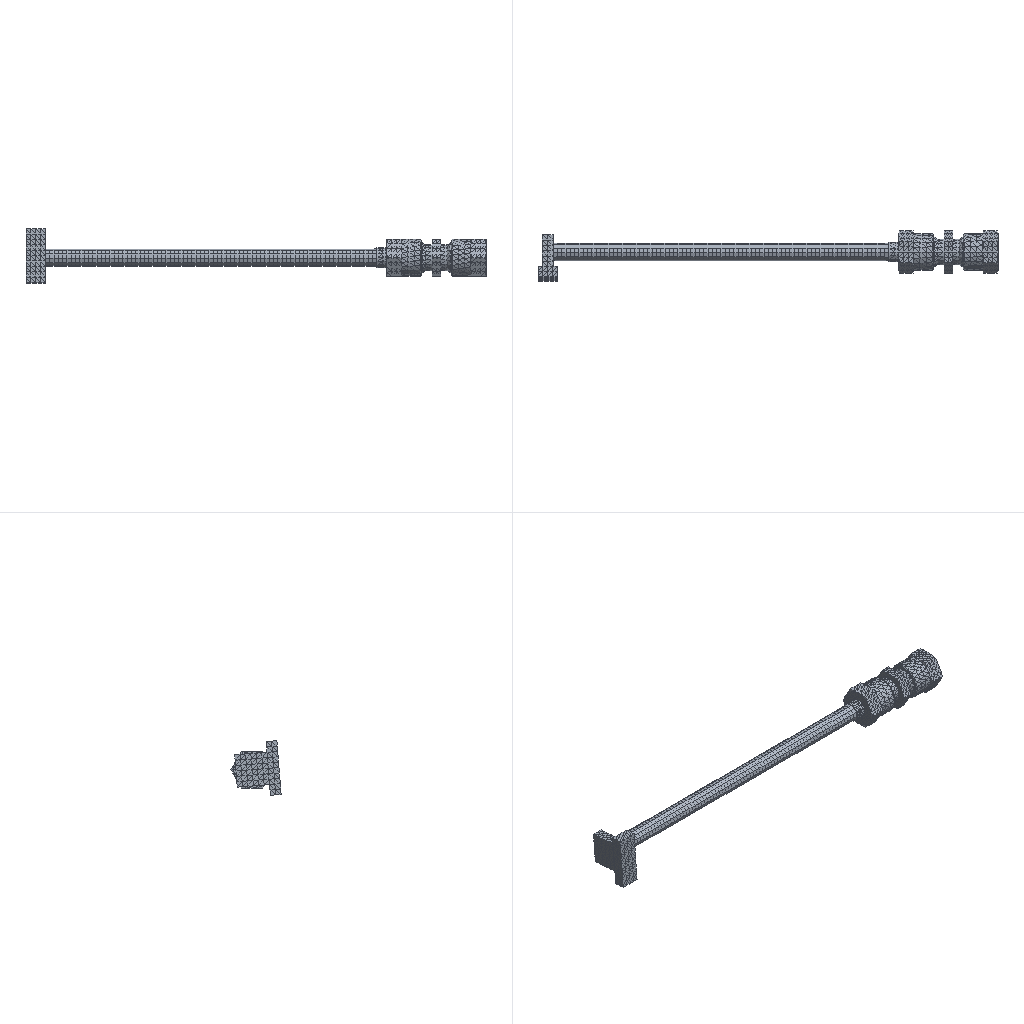Simulation study | abaqus
Set-up summary:
category,name,step,type,value,unit,region
solver,abaqus,,Abaqus/CAE 2024
units,mm-N-s-tonne (MPa),,inferred,E=106000 density=4.48e-09
analysis,Step-1,,static,time_period=1
mesh,nodes,,,14303
mesh,elements,,,7999
element_type,C3D10,,,6919
element_type,S4R,,,1080
material,dg,,E,106000
material,dg,,nu,0.3
material,dg,,density,4.48e-09
material,dg,,cte,8.3e-06
material,dg,,behaviors,expansion
material,jt,,E,119000
material,jt,,nu,0.34
material,jt,,density,4.5e-09
material,jt,,cte,8.2e-06
material,jt,,behaviors,expansion
section,jt,,solid section,,,Set-1
section,jt,,solid section,,,Set-1
section,jt,,solid section,,,Set-1
section,jt,,solid section,,,Set-1
section,jt,,solid section,,,Set-1
section,jt,,solid section,,,Set-1
section,dg,,shell section,0.54,,Set-2
load,Predefined,initial,initial condition temperature
load,Load-1,Step-1,pressure,35,,Surf-13
load,Load-2,Step-1,pressure,35,,Surf-14
load,Predefined,Step-1,temperature,50,,Set-2
bc,BC-1,Step-1,encastre,[dofs=ENCASTRE],,Set-1
contact,Constraint-1,initial,tie,,,s_Surf-1 / m_Surf-1
contact,Constraint-2,initial,tie,,,s_Surf-3 / m_Surf-3
contact,Constraint-3,initial,tie,,,s_Surf-5 / m_Surf-5
contact,Constraint-4,initial,tie,,,s_Surf-7 / m_Surf-7
contact,Constraint-5,initial,tie,,,s_Surf-9 / m_Surf-9
contact,Constraint-6,initial,tie,,,s_Surf-11 / m_Surf-11
Abaqus input file, long lists of numbers shortened:
*Heading
** Job name: deck Model name: Model-1
** Generated by: Abaqus/CAE 2024
*Preprint, echo=NO, model=NO, history=NO, contact=NO
**
** PARTS
**
*Part, name=dg
*End Part
**
*Part, name=gt
*Node
      1,  -21.082, -0.3744,          -6.
      2,  -15.858, -0.3744,          -6.
** (1643 more lines like these left out)
*Element, type=C3D10
  1,  245,   91,  111,   92,  286,  285,  284,  288,  287,  289
  2,  246,  245,  110,  134,  292,  291,  290,  294,  293,  295
** (815 more lines like these left out)
*Nset, nset=Set-1, generate
    1,  1645,     1
*Elset, elset=Set-1, generate
   1,  817,    1
** Section: jt
*Solid Section, elset=Set-1, material=jt
,
*End Part
**
*Part, name=jiaju
*Node
      1,  -190.749,  -13.813,  -11.485
      2,  -181.749,  -13.813,  -11.485
** (2282 more lines like these left out)
*Element, type=C3D10
   1,  119,  262,  263,  252,  368,  367,  366,  370,  369,  371
   2,  181,  262,  219,  264,  374,  373,  372,  376,  375,  377
** (1294 more lines like these left out)
*Nset, nset=Set-1, generate
    1,  2284,     1
*Elset, elset=Set-1, generate
    1,  1296,     1
** Section: jt
*Solid Section, elset=Set-1, material=jt
,
*End Part
**
*Part, name=jietouzuo
*Node
      1,  -5.749, -0.3744,  -5.95
      2,  -5.749, -0.3744,   5.95
** (1310 more lines like these left out)
*Element, type=C3D10
  1,  187,   68,  104,  166,  221,  220,  219,  223,  222,  224
  2,  187,  103,   68,   67,  226,  225,  221,  228,  227,  229
** (688 more lines like these left out)
*Nset, nset=Set-1, generate
    1,  1312,     1
*Elset, elset=Set-1, generate
   1,  690,    1
** Section: jt
*Solid Section, elset=Set-1, material=jt
,
*End Part
**
*Part, name=jtyou
*Node
      1,   10.751, -0.3744,           7.
      2,   5.751, -0.3744,           7.
** (2225 more lines like these left out)
*Element, type=C3D10
   1,  309,  287,  310,  311,  368,  367,  366,  370,  369,  371
   2,  309,  257,   15,  164,  374,  373,  372,  376,  375,  377
** (1187 more lines like these left out)
*Nset, nset=Set-1, generate
    1,  2227,     1
*Elset, elset=Set-1, generate
    1,  1189,     1
** Section: jt
*Solid Section, elset=Set-1, material=jt
,
*End Part
**
*Part, name=lmyou
*Node
      1,   22.11, -0.3744,        4.625
      2,   22.11, -0.3744,       -4.625
** (2978 more lines like these left out)
*Element, type=C3D10
   1,  460,  461,   79,  295,  499,  498,  497,  501,  500,  502
   2,  460,  462,  276,   80,  505,  504,  503,  507,  506,  508
** (1530 more lines like these left out)
*Nset, nset=Set-1, generate
    1,  2980,     1
*Elset, elset=Set-1, generate
    1,  1532,     1
** Section: jt
*Solid Section, elset=Set-1, material=jt
,
*End Part
**
*Part, name=lmzuo
*Node
      1,  -23.607, -0.3744,        4.625
      2,  -23.607, -0.3744,       -4.625
** (2761 more lines like these left out)
*Element, type=C3D10
   1,  435,  436,   94,  279,  470,  469,  468,  472,  471,  473
   2,  162,  308,  200,  437,  476,  475,  474,  478,  477,  479
** (1393 more lines like these left out)
*Nset, nset=Set-1, generate
    1,  2763,     1
*Elset, elset=Set-1, generate
    1,  1395,     1
** Section: jt
*Solid Section, elset=Set-1, material=jt
,
*End Part
**
**
** ASSEMBLY
**
*Assembly, name=Assembly
**
*Instance, name=dg-1, part=dg
*Node
      1,  -12.308, -0.7027,   3.986
      2,  -12.308, -0.046,  -3.986
** (1090 more lines like these left out)
*Element, type=S4R
 1,   1,  11, 233,  22
 2,  11,  12, 234, 233
** (1078 more lines like these left out)
*Nset, nset=Set-2, generate
    1,  1092,     1
*Elset, elset=Set-2, generate
    1,  1080,     1
** Section: dg
*Shell Section, elset=Set-2, material=dg, offset=SPOS
0.54, 5
*End Instance
**
*Instance, name=gt-1, part=gt
*End Instance
**
*Instance, name=jiaju-1, part=jiaju
*End Instance
**
*Instance, name=jietouzuo-1, part=jietouzuo
*End Instance
**
*Instance, name=jtyou-1, part=jtyou
*End Instance
**
*Instance, name=lmyou-1, part=lmyou
*End Instance
**
*Instance, name=lmzuo-1, part=lmzuo
*End Instance
**
*Nset, nset=Set-1, instance=jiaju-1
    1,    2,    3,    4,   21,   22,   23,   24,   25,   26,   27,   28,   29,   30,   31,   32
   33,   34,   35,   36,   37,   38,   39,   40,   41,   42,   43,   44,  135,  136,  137,  138
** (10 more lines like these left out)
*Elset, elset=Set-1, instance=jiaju-1
   29,   42,   79,   80,  112,  129,  168,  207,  242,  266,  271,  274,  284,  297,  300,  331
  341,  356,  399,  416,  446,  448,  464,  493,  531,  592,  631,  640,  691,  693,  697,  712
** (3 more lines like these left out)
*Nset, nset=Set-2, instance=dg-1, generate
    1,  1092,     1
*Nset, nset=Set-2, instance=gt-1, generate
    1,  1645,     1
*Nset, nset=Set-2, instance=jietouzuo-1, generate
    1,  1312,     1
*Nset, nset=Set-2, instance=lmyou-1, generate
    1,  2980,     1
*Nset, nset=Set-2, instance=jiaju-1, generate
    1,  2284,     1
*Nset, nset=Set-2, instance=jtyou-1, generate
    1,  2227,     1
*Elset, elset=Set-2, instance=dg-1, generate
    1,  1080,     1
*Elset, elset=Set-2, instance=gt-1, generate
   1,  817,    1
*Elset, elset=Set-2, instance=jietouzuo-1, generate
   1,  690,    1
*Elset, elset=Set-2, instance=lmyou-1, generate
    1,  1532,     1
*Elset, elset=Set-2, instance=jiaju-1, generate
    1,  1296,     1
*Elset, elset=Set-2, instance=jtyou-1, generate
    1,  1189,     1
*Nset, nset=Set-3, instance=dg-1, generate
    1,  1092,     1
*Nset, nset=Set-3, instance=gt-1, generate
    1,  1645,     1
*Nset, nset=Set-3, instance=jietouzuo-1, generate
    1,  1312,     1
*Nset, nset=Set-3, instance=lmyou-1, generate
    1,  2980,     1
*Nset, nset=Set-3, instance=jiaju-1, generate
    1,  2284,     1
*Nset, nset=Set-3, instance=jtyou-1, generate
    1,  2227,     1
*Elset, elset=Set-3, instance=dg-1, generate
    1,  1080,     1
*Elset, elset=Set-3, instance=gt-1, generate
   1,  817,    1
*Elset, elset=Set-3, instance=jietouzuo-1, generate
   1,  690,    1
*Elset, elset=Set-3, instance=lmyou-1, generate
    1,  1532,     1
*Elset, elset=Set-3, instance=jiaju-1, generate
    1,  1296,     1
*Elset, elset=Set-3, instance=jtyou-1, generate
    1,  1189,     1
*Elset, elset=_Surf-13_SNEG, internal, instance=dg-1, generate
    1,  1080,     1
*Surface, type=ELEMENT, name=Surf-13
_Surf-13_SNEG, SNEG
*Elset, elset=_Surf-14_S3, internal, instance=jietouzuo-1
  26,  52,  83,  91, 127, 192, 202, 304, 406, 438, 542, 565, 566, 574, 581, 585
 586, 589, 591, 592, 598, 620, 666, 668, 689
*Elset, elset=_Surf-14_S3, internal, instance=jtyou-1
   19,   20,  177,  207,  227,  350,  353,  361,  400,  421,  499,  505,  513,  515,  523,  524
  526,  536,  553,  561,  562,  578,  596,  598,  675,  688,  691,  768,  872,  944,  993, 1002
** (1 more lines like these left out)
*Elset, elset=_Surf-14_S2, internal, instance=jietouzuo-1
 432, 434, 482, 634, 637
*Elset, elset=_Surf-14_S2, internal, instance=jtyou-1
  238,  482,  597,  721,  725,  771, 1136, 1181
*Elset, elset=_Surf-14_S4, internal, instance=jietouzuo-1
 535,
*Elset, elset=_Surf-14_S4, internal, instance=jtyou-1
  289,  415,  425,  504,  551,  552,  554,  574,  603,  971,  983, 1095
*Elset, elset=_Surf-14_S1, internal, instance=jietouzuo-1
 416,
*Elset, elset=_Surf-14_S1, internal, instance=jtyou-1
  516,  518,  713,  758,  831, 1093, 1119, 1122
*Surface, type=ELEMENT, name=Surf-14
_Surf-14_S3, S3
_Surf-14_S2, S2
_Surf-14_S4, S4
_Surf-14_S1, S1
*Elset, elset=_m_Surf-1_S3, internal, instance=jiaju-1
  101,  110,  375,  435,  472,  522,  620,  723,  730,  746,  750,  752,  756,  764,  774,  779
  825,  831,  892,  957,  992, 1182
*Elset, elset=_m_Surf-1_S2, internal, instance=jiaju-1
  114,  731,  771,  800,  832, 1128
*Elset, elset=_m_Surf-1_S1, internal, instance=jiaju-1
    5,  188,  776,  777,  787,  812,  933, 1035, 1199
*Elset, elset=_m_Surf-1_S4, internal, instance=jiaju-1
  790,  983, 1065
*Surface, type=ELEMENT, name=m_Surf-1
_m_Surf-1_S3, S3
_m_Surf-1_S2, S2
_m_Surf-1_S4, S4
_m_Surf-1_S1, S1
*Elset, elset=_m_Surf-3_S1, internal, instance=lmzuo-1
   63,  177,  209,  214,  243,  269,  295,  301,  379,  396,  441,  453,  462,  471,  497,  502
  519,  534,  543,  560,  569,  579,  590,  594,  607,  628,  664,  679,  688,  706,  708,  785
** (1 more lines like these left out)
*Elset, elset=_m_Surf-3_S4, internal, instance=lmzuo-1
  213,  265,  267,  279,  300,  312,  361,  430,  447,  459,  460,  492,  512,  516,  518,  523
  531,  538,  539,  549,  552,  558,  559,  565,  566,  567,  606,  641,  657,  701,  714,  743
** (1 more lines like these left out)
*Elset, elset=_m_Surf-3_S2, internal, instance=lmzuo-1
  197,  227,  235,  247,  284,  286,  299,  330,  350,  424,  439,  456,  465,  489,  520,  581
  585,  597,  608,  609,  610,  617,  622,  626,  635,  687,  700,  709,  720,  754,  767,  801
** (1 more lines like these left out)
*Elset, elset=_m_Surf-3_S3, internal, instance=lmzuo-1
  184,  296,  318,  336,  340,  353,  390,  393,  394,  403,  404,  405,  406,  423,  428,  436
  446,  450,  467,  470,  475,  480,  483,  490,  499,  507,  550,  551,  573,  574,  587,  598
** (2 more lines like these left out)
*Surface, type=ELEMENT, name=m_Surf-3
_m_Surf-3_S1, S1
_m_Surf-3_S4, S4
_m_Surf-3_S2, S2
_m_Surf-3_S3, S3
*Elset, elset=_m_Surf-5_S3, internal, instance=lmyou-1
   74,  253,  254,  260,  262,  330,  334,  345,  364,  368,  375,  382,  416,  422,  432,  439
  440,  447,  452,  457,  461,  508,  560,  562,  573,  590,  591,  599,  602,  679,  681,  708
** (1 more lines like these left out)
*Elset, elset=_m_Surf-5_S2, internal, instance=lmyou-1
  247,  276,  279,  307,  309,  366,  373,  398,  413,  417,  418,  453,  466,  472,  474,  480
  485,  498,  506,  523,  540,  545,  567,  570,  575,  576,  611,  631,  639,  664,  754,  765
** (1 more lines like these left out)
*Elset, elset=_m_Surf-5_S4, internal, instance=lmyou-1
  255,  264,  311,  326,  333,  377,  378,  384,  389,  391,  393,  406,  410,  411,  423,  437
  442,  454,  460,  467,  479,  487,  489,  494,  510,  512,  527,  533,  539,  549,  574,  589
** (2 more lines like these left out)
*Elset, elset=_m_Surf-5_S1, internal, instance=lmyou-1
   82,  207,  244,  267,  275,  290,  337,  342,  347,  394,  455,  491,  502,  505,  513,  518
  526,  535,  544,  565,  566,  569,  578,  582,  588,  675,  734,  750,  789,  841,  867,  907
** (1 more lines like these left out)
*Surface, type=ELEMENT, name=m_Surf-5
_m_Surf-5_S3, S3
_m_Surf-5_S2, S2
_m_Surf-5_S4, S4
_m_Surf-5_S1, S1
*Elset, elset=_m_Surf-7_S4, internal, instance=jietouzuo-1
  14,  48, 177, 204, 285, 291, 324
*Elset, elset=_m_Surf-7_S3, internal, instance=jietouzuo-1
  21,  74,  85, 156, 173, 185, 206, 235, 240, 242, 244, 252, 298, 300, 306, 339
 362, 408, 452, 604, 622
*Elset, elset=_m_Surf-7_S1, internal, instance=jietouzuo-1
  30, 258, 316, 331
*Elset, elset=_m_Surf-7_S2, internal, instance=jietouzuo-1
 241, 325, 357, 522
*Surface, type=ELEMENT, name=m_Surf-7
_m_Surf-7_S4, S4
_m_Surf-7_S3, S3
_m_Surf-7_S2, S2
_m_Surf-7_S1, S1
*Elset, elset=_m_Surf-9_S2, internal, instance=gt-1
   3,  46,  60,  65, 109, 113, 123, 135, 157, 172, 176, 199, 203, 208, 231, 240
 244, 259, 315, 321, 348, 367, 380, 383, 398, 573, 592, 644
*Elset, elset=_m_Surf-9_S4, internal, instance=gt-1
   4,  17,  40,  70,  72,  95, 100, 107, 130, 133, 137, 161, 221, 224, 238, 239
 264, 290, 303, 330, 392, 407, 425, 427, 475, 485, 543, 657, 675, 697, 704, 710
** (1 more lines like these left out)
*Elset, elset=_m_Surf-9_S1, internal, instance=gt-1
  27,  47,  48,  53,  61,  71,  87,  92, 110, 163, 167, 194, 204, 212, 226, 229
 233, 242, 243, 253, 267, 308, 399, 402, 441, 445, 591, 667, 684, 688, 726
*Elset, elset=_m_Surf-9_S3, internal, instance=gt-1
  34,  42,  58,  84,  96, 105, 126, 140, 153, 162, 170, 180, 183, 191, 200, 213
 214, 230, 249, 260, 295, 325, 338, 451, 629, 680, 683, 706
*Surface, type=ELEMENT, name=m_Surf-9
_m_Surf-9_S2, S2
_m_Surf-9_S4, S4
_m_Surf-9_S1, S1
_m_Surf-9_S3, S3
*Elset, elset=_m_Surf-11_S3, internal, instance=jtyou-1
   59,   81,  127,  135,  170,  174,  190,  254,  277,  282,  285,  297,  298,  303,  341,  346
  351,  374,  406,  416,  428,  433,  435,  440,  448,  449,  452,  460,  465,  482,  493,  503
** (2 more lines like these left out)
*Elset, elset=_m_Surf-11_S2, internal, instance=jtyou-1
  148,  330,  453,  479,  487,  553,  641,  702,  829,  943,  944, 1064
*Elset, elset=_m_Surf-11_S1, internal, instance=jtyou-1
  195,  414,  476,  576,  608,  627,  652,  692, 1168
*Elset, elset=_m_Surf-11_S4, internal, instance=jtyou-1
  387,  446,  455,  494,  505,  520,  536,  566,  632,  651,  653,  670,  695,  735,  968, 1068
*Surface, type=ELEMENT, name=m_Surf-11
_m_Surf-11_S3, S3
_m_Surf-11_S2, S2
_m_Surf-11_S4, S4
_m_Surf-11_S1, S1
*Elset, elset=_s_Surf-1_SPOS, internal, instance=dg-1
 1009, 1010, 1011, 1012, 1013, 1014, 1015, 1016, 1017, 1018, 1019, 1020, 1069, 1070, 1071, 1072
 1073, 1074, 1075, 1076, 1077, 1078, 1079, 1080
*Surface, type=ELEMENT, name=s_Surf-1
_s_Surf-1_SPOS, SPOS
*Elset, elset=_s_Surf-3_S4, internal, instance=jietouzuo-1
   9, 172, 284, 377, 541
*Elset, elset=_s_Surf-3_S3, internal, instance=jietouzuo-1
  60,  65,  66,  97, 107, 110, 111, 129, 134, 149, 151, 178, 181, 205, 261, 272
 278, 327, 332, 340, 343, 369, 371, 404, 428, 431, 436, 444, 465, 466, 473, 480
** (2 more lines like these left out)
*Elset, elset=_s_Surf-3_S1, internal, instance=jietouzuo-1
 157, 174, 247, 260, 262, 269, 472, 494, 627
*Elset, elset=_s_Surf-3_S2, internal, instance=jietouzuo-1
 280, 330, 451, 471, 484, 503
*Surface, type=ELEMENT, name=s_Surf-3
_s_Surf-3_S4, S4
_s_Surf-3_S3, S3
_s_Surf-3_S2, S2
_s_Surf-3_S1, S1
*Elset, elset=_s_Surf-5_S3, internal, instance=jtyou-1
   66,   70,   71,   75,   80,  116,  122,  143,  167,  185,  215,  311,  386,  443,  450,  462
  466,  484,  490,  529,  543,  546,  560,  589,  591,  611,  615,  630,  646,  722,  727,  744
** (2 more lines like these left out)
*Elset, elset=_s_Surf-5_S1, internal, instance=jtyou-1
 137,
*Elset, elset=_s_Surf-5_S4, internal, instance=jtyou-1
  161,  846,  991, 1189
*Elset, elset=_s_Surf-5_S2, internal, instance=jtyou-1
  837,  866, 1129, 1179
*Surface, type=ELEMENT, name=s_Surf-5
_s_Surf-5_S3, S3
_s_Surf-5_S1, S1
_s_Surf-5_S4, S4
_s_Surf-5_S2, S2
*Elset, elset=_s_Surf-7_S3, internal, instance=gt-1
  33,  39, 247, 316, 369, 377
*Elset, elset=_s_Surf-7_S4, internal, instance=gt-1
   8,  28,  37, 252, 255, 553, 586, 672
*Elset, elset=_s_Surf-7_S2, internal, instance=gt-1
 256, 261, 287, 305, 313, 462, 590
*Elset, elset=_s_Surf-7_S1, internal, instance=gt-1
  29, 699, 715
*Surface, type=ELEMENT, name=s_Surf-7
_s_Surf-7_S3, S3
_s_Surf-7_S4, S4
_s_Surf-7_S2, S2
_s_Surf-7_S1, S1
*Elset, elset=_s_Surf-9_SPOS, internal, instance=dg-1
   13,   14,   15,   16,   17,   18,   19,   20,   21,   22,   23,   24,   25,   26,   27,   28
   29,   30,   31,   32,   33,   34,   35,   36,   37,   38,   39,   40,   41,   42,   43,   44
** (4 more lines like these left out)
*Surface, type=ELEMENT, name=s_Surf-9
_s_Surf-9_SPOS, SPOS
*Elset, elset=_s_Surf-11_S4, internal, instance=jietouzuo-1
  25, 672
*Elset, elset=_s_Surf-11_S3, internal, instance=jietouzuo-1
  27,  33, 131, 164, 478, 551, 552, 553, 557, 558, 559, 599, 600, 615, 650, 654
 656, 660, 662, 663, 664, 670, 681
*Elset, elset=_s_Surf-11_S2, internal, instance=jietouzuo-1
 474,
*Surface, type=ELEMENT, name=s_Surf-11
_s_Surf-11_S4, S4
_s_Surf-11_S3, S3
_s_Surf-11_S2, S2
** Constraint: Constraint-1
*Tie, name=Constraint-1, adjust=yes
s_Surf-1, m_Surf-1
** Constraint: Constraint-2
*Tie, name=Constraint-2, adjust=yes
s_Surf-3, m_Surf-3
** Constraint: Constraint-3
*Tie, name=Constraint-3, adjust=yes
s_Surf-5, m_Surf-5
** Constraint: Constraint-4
*Tie, name=Constraint-4, adjust=yes
s_Surf-7, m_Surf-7
** Constraint: Constraint-5
*Tie, name=Constraint-5, adjust=yes
s_Surf-9, m_Surf-9
** Constraint: Constraint-6
*Tie, name=Constraint-6, adjust=yes
s_Surf-11, m_Surf-11
*End Assembly
**
** MATERIALS
**
*Material, name=dg
*Density
 4.48e-09,
*Elastic
106000., 0.3,-55.
104500., 0.3,-20.
103500., 0.3,  0.
101500., 0.3, 50.
 98000., 0.3,100.
 96000., 0.3,120.
 94500., 0.3,135.
 93500., 0.3,145.
 92500., 0.3,155.
 91500., 0.3,165.
 90500., 0.3,175.
 89500., 0.3,185.
 88500., 0.3,195.
 87500., 0.3,205.
 86500., 0.3,215.
 85500., 0.3,225.
 84500., 0.3,235.
*Expansion, zero=20.
 8.3e-06,-55.
 8.6e-06,-20.
 8.7e-06,  0.
 8.7e-06, 50.
 8.7e-06,100.
 9.2e-06,120.
 9.2e-06,135.
 9.2e-06,145.
 9.2e-06,155.
 9.2e-06,165.
 9.2e-06,175.
 9.2e-06,185.
 9.2e-06,195.
 9.2e-06,205.
 9.2e-06,215.
 9.2e-06,225.
 9.2e-06,235.
*Material, name=jt
*Density
 4.5e-09,
*Elastic
119000., 0.34, -55.
117500., 0.34, -20.
116500., 0.34,   0.
114500., 0.34,  50.
112500., 0.34, 100.
111500., 0.34, 120.
110800., 0.34, 135.
110200., 0.34, 145.
109600., 0.34, 155.
109000., 0.34, 165.
108300., 0.34, 175.
107600., 0.34, 185.
106900., 0.34, 195.
106200., 0.34, 205.
105500., 0.34, 215.
104800., 0.34, 225.
104100., 0.34, 235.
*Expansion
  8.2e-06,-55.
  8.5e-06,-20.
  8.7e-06,  0.
  8.9e-06, 50.
    9e-06,100.
  9.1e-06,120.
 9.15e-06,135.
  9.2e-06,145.
 9.25e-06,155.
  9.3e-06,165.
 9.35e-06,175.
  9.4e-06,185.
 9.45e-06,195.
  9.5e-06,205.
 9.55e-06,215.
  9.6e-06,225.
 9.65e-06,235.
**
** PREDEFINED FIELDS
**
** Name: Predefined Field-1   Type: Temperature
*Initial Conditions, type=TEMPERATURE
Set-2, 20.
** ----------------------------------------------------------------
**
** STEP: Step-1
**
*Step, name=Step-1, nlgeom=NO
*Static
0.01, 1., 1e-05, 0.1
**
** BOUNDARY CONDITIONS
**
** Name: BC-1 Type: Symmetry/Antisymmetry/Encastre
*Boundary
Set-1, ENCASTRE
**
** LOADS
**
** Name: Load-1   Type: Pressure
*Dsload
Surf-13, P, 35.
** Name: Load-2   Type: Pressure
*Dsload
Surf-14, P, 35.
**
** PREDEFINED FIELDS
**
** Name: Predefined Field-1   Type: Temperature
*Temperature
Set-2, 50.
**
** OUTPUT REQUESTS
**
*Restart, write, frequency=0
**
** FIELD OUTPUT: F-Output-1
**
*Output, field
*Node Output
U, UR, UT, V, VR, VT
*Element Output, directions=YES
E, EE, EEQUT, ER, IE, LE, NE, PE, PEEQ, PEEQMAX, PEEQT, PEMAG, PEQC, S, SALPHA, SE
SEE, SEP, SEPE, SPE, TE, TEEQ, TEVOL, THE, VE, VEEQ
**
** HISTORY OUTPUT: H-Output-1
**
*Output, history, variable=PRESELECT
*End Step
Results summary:
result,odb.job_status,,,JOB_STATUS_COMPLETED_SUCCESSFULLY,"consistent, unstated (Abaqus has no unit system)"
result,steps[0].procedure,Step-1,,*STATIC,"consistent, unstated (Abaqus has no unit system)"
result,steps[0].time_period,Step-1,,1,"consistent, unstated (Abaqus has no unit system)"
result,steps[0].n_frames,Step-1,,16,"consistent, unstated (Abaqus has no unit system)"
result,steps[0].last_frame.id,Step-1,,15,"consistent, unstated (Abaqus has no unit system)"
result,steps[0].last_frame.value,Step-1,,1,"consistent, unstated (Abaqus has no unit system)"
result,steps[0].last_frame.description,Step-1,,Increment     15: Step Time =    1.000,"consistent, unstated (Abaqus has no unit system)"
result,steps[0].completed,Step-1,,True,"consistent, unstated (Abaqus has no unit system)"
result,steps[0].max_U_magnitude,Step-1,,0.08626,"consistent, unstated (Abaqus has no unit system)"
result,steps[0].max_S_mises,Step-1,,307.2,"consistent, unstated (Abaqus has no unit system)"